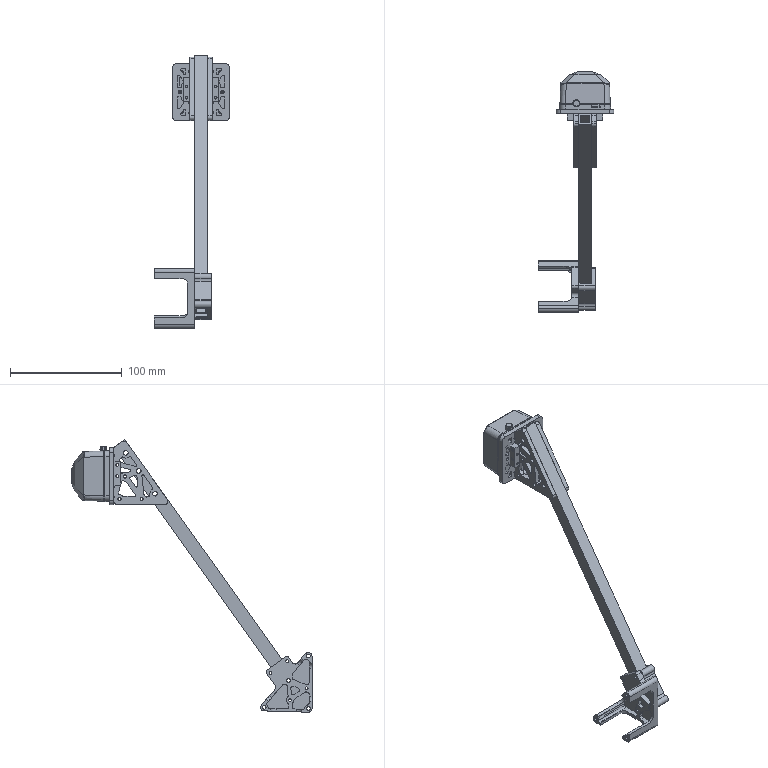Part | SolidWorks | 14 solids | 1140 faces | box 67.75 x 214.75 x 243.725 mm | volume 76567 mm3 | cylinder 537 | plane 523 | spline 53 | cone 27 | commonest cylinder face diameters 2.5 x87 2.2 x72 2 x40 2.1 x36 4 x33 4.1 x26